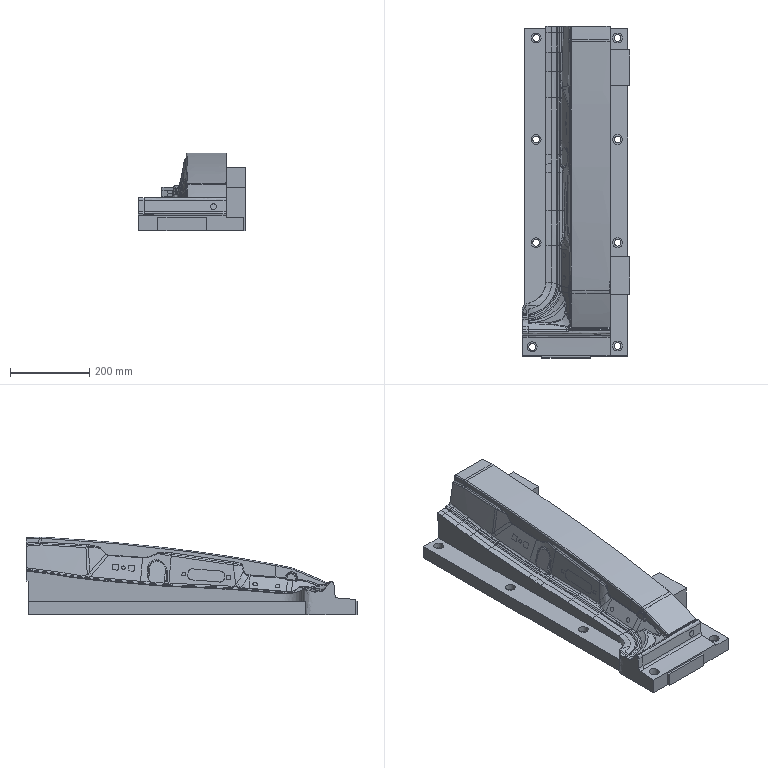Part | NX | features solid 2 | 1 solid | 348 faces | box 271.276 x 835 x 196.106 mm | volume 16649381 mm3 | spline 192 | plane 72 | cylinder 72 | sphere 12 | commonest cylinder face diameters 10 x13 6.001 x10 17 x8 25 x8 6.004 x3 11.101 x3